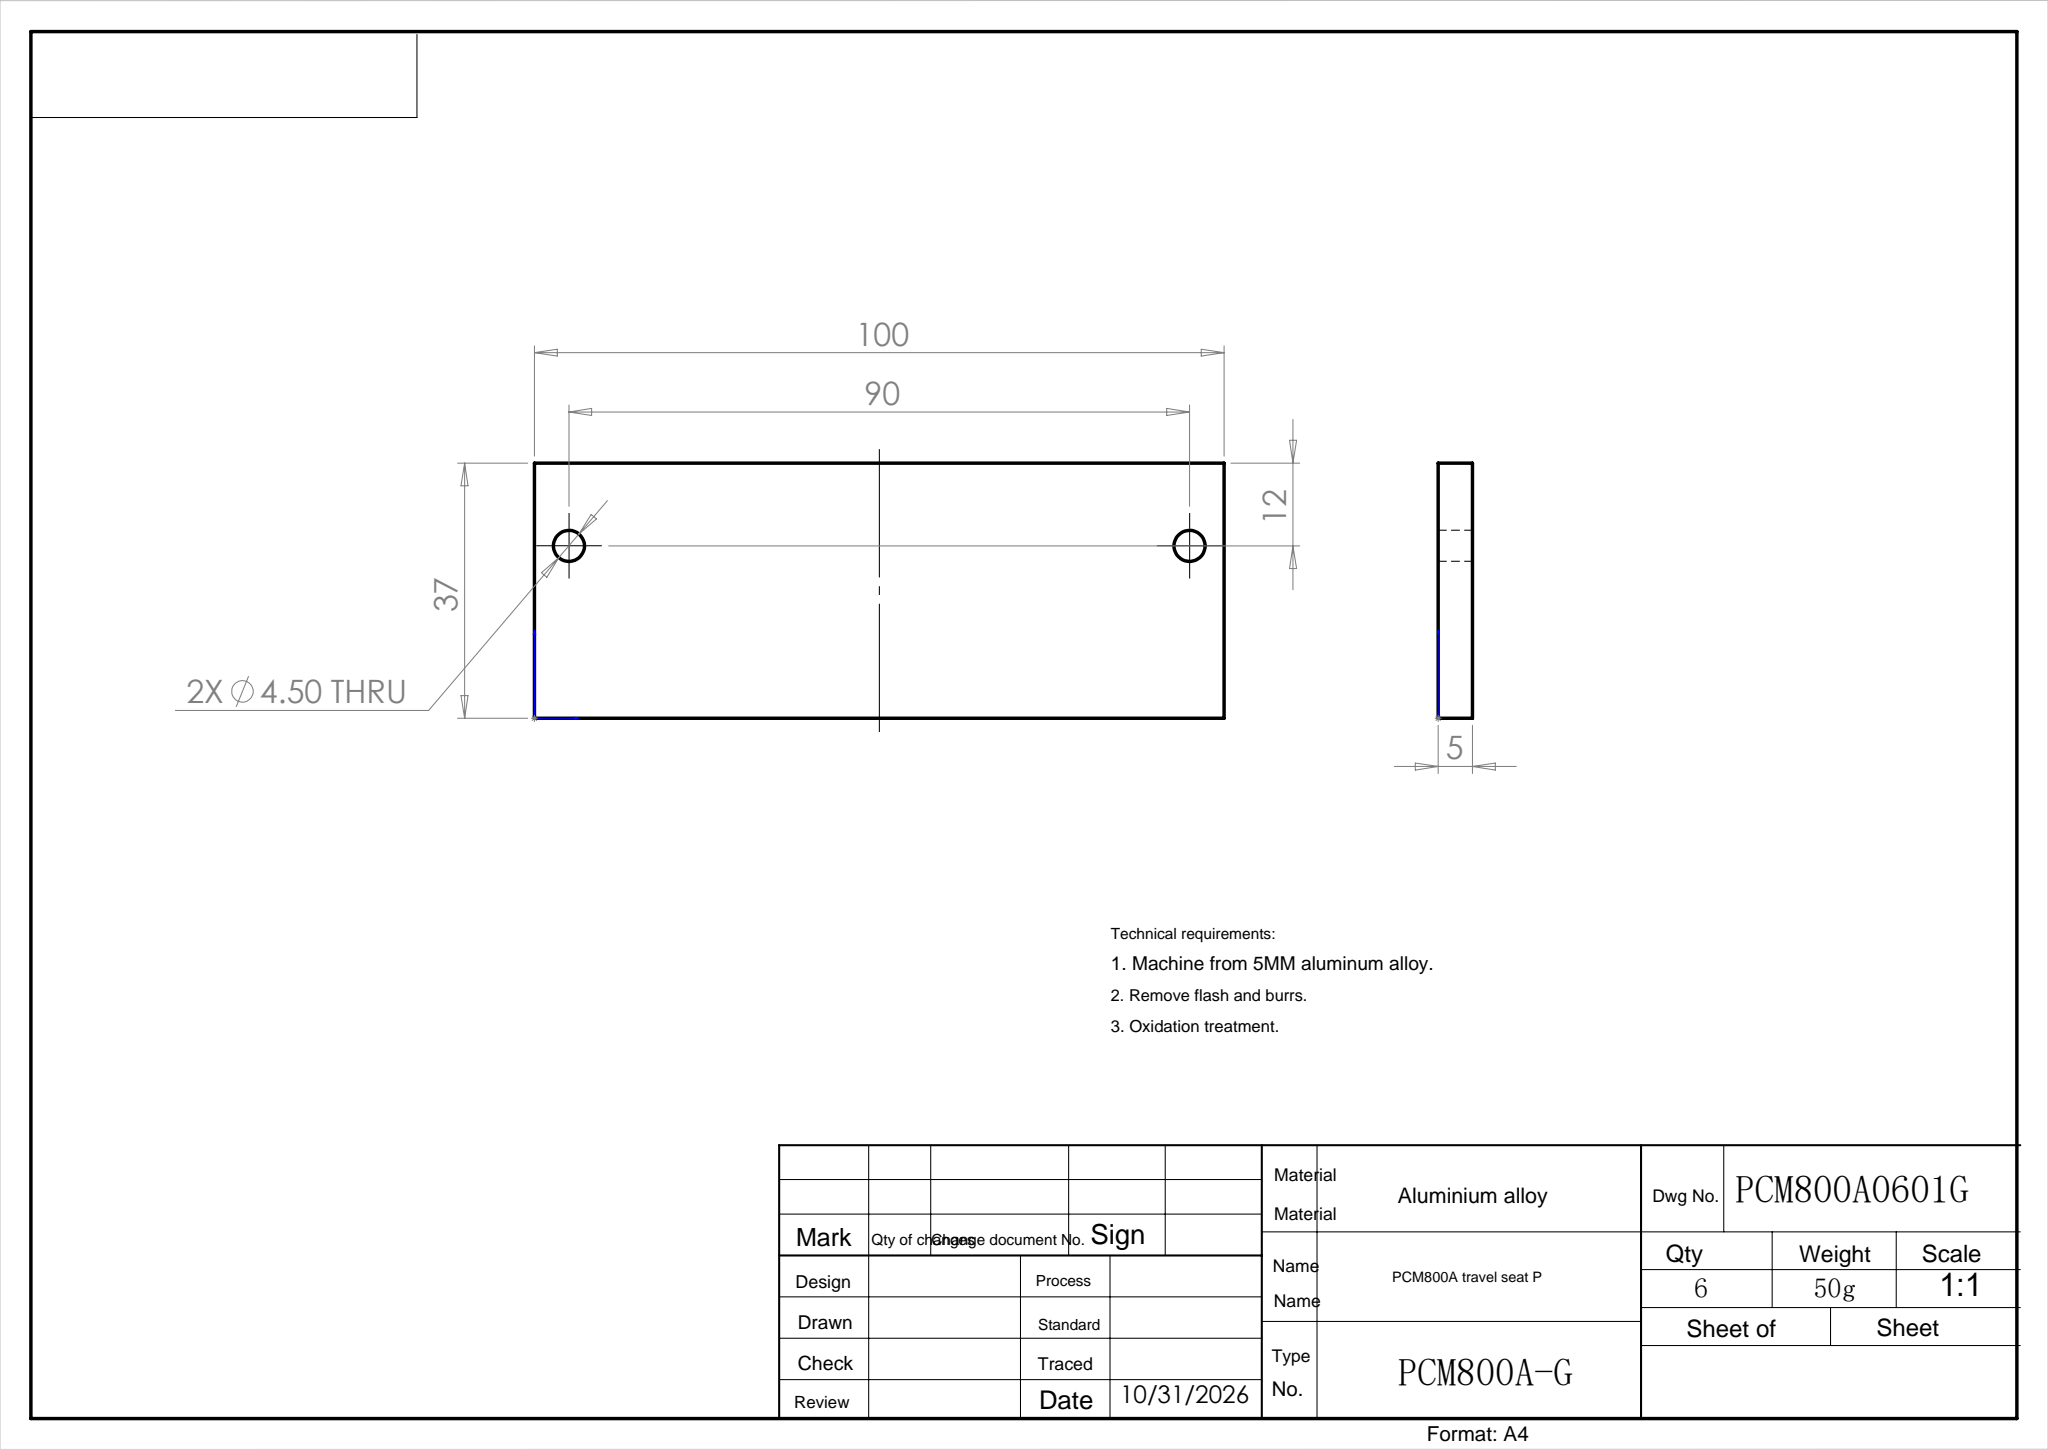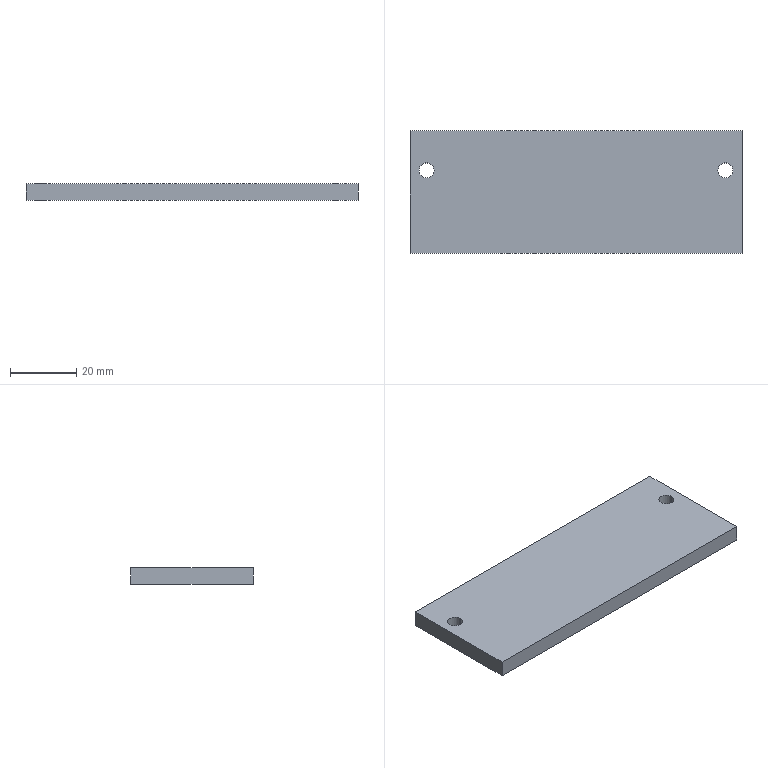Part | SolidWorks | features Extrusion 1, ICE 1 | 1 solid | 10 faces | box 100 x 37 x 5 mm | volume 18341 mm3 | plane 6 | cylinder 4 | commonest cylinder face diameters 4.5 x4
STEP:
#1=CARTESIAN_POINT('',(92.75,25.,0.));
#2=VERTEX_POINT('',#1);
#3=CARTESIAN_POINT('',(97.25,25.,0.));
#4=VERTEX_POINT('',#3);
#5=CARTESIAN_POINT('',(95.,25.,0.));
#6=DIRECTION('',(0.,0.,1.));
#7=DIRECTION('',(1.,0.,0.));
#8=AXIS2_PLACEMENT_3D('',#5,#6,#7);
#9=CIRCLE('',#8,2.25);
#10=EDGE_CURVE('',#2,#4,#9,.T.);
#11=ORIENTED_EDGE('',*,*,#10,.F.);
#12=CARTESIAN_POINT('',(92.75,25.,5.));
#13=VERTEX_POINT('',#12);
#14=CARTESIAN_POINT('',(92.75,25.,0.));
#15=DIRECTION('',(0.,0.,1.));
#16=VECTOR('',#15,1000.);
#17=LINE('',#14,#16);
#18=EDGE_CURVE('',#2,#13,#17,.T.);
#19=ORIENTED_EDGE('',*,*,#18,.T.);
#20=CARTESIAN_POINT('',(97.25,25.,5.));
#21=VERTEX_POINT('',#20);
#22=CARTESIAN_POINT('',(95.,25.,5.));
#23=DIRECTION('',(0.,0.,1.));
#24=DIRECTION('',(1.,0.,0.));
#25=AXIS2_PLACEMENT_3D('',#22,#23,#24);
#26=CIRCLE('',#25,2.25);
#27=EDGE_CURVE('',#13,#21,#26,.T.);
#28=ORIENTED_EDGE('',*,*,#27,.T.);
#29=CARTESIAN_POINT('',(97.25,25.,0.));
#30=DIRECTION('',(0.,0.,1.));
#31=VECTOR('',#30,1000.);
#32=LINE('',#29,#31);
#33=EDGE_CURVE('',#4,#21,#32,.T.);
#34=ORIENTED_EDGE('',*,*,#33,.F.);
#35=EDGE_LOOP('',(#11,#19,#28,#34));
#36=FACE_OUTER_BOUND('',#35,.T.);
#37=CARTESIAN_POINT('',(95.,25.,0.));
#38=DIRECTION('',(0.,0.,1.));
#39=DIRECTION('',(1.,0.,0.));
#40=AXIS2_PLACEMENT_3D('',#37,#38,#39);
#41=CYLINDRICAL_SURFACE('',#40,2.25);
#42=ADVANCED_FACE('',(#36),#41,.F.);
#43=CARTESIAN_POINT('',(2.75,25.,0.));
#44=VERTEX_POINT('',#43);
#45=CARTESIAN_POINT('',(7.25,25.,0.));
#46=VERTEX_POINT('',#45);
#47=CARTESIAN_POINT('',(5.,25.,0.));
#48=DIRECTION('',(0.,0.,1.));
#49=DIRECTION('',(1.,0.,0.));
#50=AXIS2_PLACEMENT_3D('',#47,#48,#49);
#51=CIRCLE('',#50,2.25);
#52=EDGE_CURVE('',#44,#46,#51,.T.);
#53=ORIENTED_EDGE('',*,*,#52,.F.);
#54=CARTESIAN_POINT('',(2.75,25.,5.));
#55=VERTEX_POINT('',#54);
#56=CARTESIAN_POINT('',(2.75,25.,0.));
#57=DIRECTION('',(0.,0.,1.));
#58=VECTOR('',#57,1000.);
#59=LINE('',#56,#58);
#60=EDGE_CURVE('',#44,#55,#59,.T.);
#61=ORIENTED_EDGE('',*,*,#60,.T.);
#62=CARTESIAN_POINT('',(7.25,25.,5.));
#63=VERTEX_POINT('',#62);
#64=CARTESIAN_POINT('',(5.,25.,5.));
#65=DIRECTION('',(0.,0.,1.));
#66=DIRECTION('',(1.,0.,0.));
#67=AXIS2_PLACEMENT_3D('',#64,#65,#66);
#68=CIRCLE('',#67,2.25);
#69=EDGE_CURVE('',#55,#63,#68,.T.);
#70=ORIENTED_EDGE('',*,*,#69,.T.);
#71=CARTESIAN_POINT('',(7.25,25.,0.));
#72=DIRECTION('',(0.,0.,1.));
#73=VECTOR('',#72,1000.);
#74=LINE('',#71,#73);
#75=EDGE_CURVE('',#46,#63,#74,.T.);
#76=ORIENTED_EDGE('',*,*,#75,.F.);
#77=EDGE_LOOP('',(#53,#61,#70,#76));
#78=FACE_OUTER_BOUND('',#77,.T.);
#79=CARTESIAN_POINT('',(5.,25.,0.));
#80=DIRECTION('',(0.,0.,1.));
#81=DIRECTION('',(1.,0.,0.));
#82=AXIS2_PLACEMENT_3D('',#79,#80,#81);
#83=CYLINDRICAL_SURFACE('',#82,2.25);
#84=ADVANCED_FACE('',(#78),#83,.F.);
#85=CARTESIAN_POINT('',(0.,37.,0.));
#86=VERTEX_POINT('',#85);
#87=CARTESIAN_POINT('',(0.,0.,0.));
#88=VERTEX_POINT('',#87);
#89=CARTESIAN_POINT('',(0.,0.,0.));
#90=DIRECTION('',(0.,-1.,0.));
#91=VECTOR('',#90,1000.);
#92=LINE('',#89,#91);
#93=EDGE_CURVE('',#86,#88,#92,.T.);
#94=ORIENTED_EDGE('',*,*,#93,.T.);
#95=CARTESIAN_POINT('',(0.,0.,5.));
#96=VERTEX_POINT('',#95);
#97=CARTESIAN_POINT('',(0.,0.,5.));
#98=DIRECTION('',(0.,0.,-1.));
#99=VECTOR('',#98,1000.);
#100=LINE('',#97,#99);
#101=EDGE_CURVE('',#96,#88,#100,.T.);
#102=ORIENTED_EDGE('',*,*,#101,.F.);
#103=CARTESIAN_POINT('',(0.,37.,5.));
#104=VERTEX_POINT('',#103);
#105=CARTESIAN_POINT('',(0.,0.,5.));
#106=DIRECTION('',(0.,-1.,0.));
#107=VECTOR('',#106,1000.);
#108=LINE('',#105,#107);
#109=EDGE_CURVE('',#104,#96,#108,.T.);
#110=ORIENTED_EDGE('',*,*,#109,.F.);
#111=CARTESIAN_POINT('',(0.,37.,5.));
#112=DIRECTION('',(0.,0.,-1.));
#113=VECTOR('',#112,1000.);
#114=LINE('',#111,#113);
#115=EDGE_CURVE('',#104,#86,#114,.T.);
#116=ORIENTED_EDGE('',*,*,#115,.T.);
#117=EDGE_LOOP('',(#94,#102,#110,#116));
#118=FACE_OUTER_BOUND('',#117,.T.);
#119=CARTESIAN_POINT('',(0.,0.,5.));
#120=DIRECTION('',(1.,0.,0.));
#121=DIRECTION('',(0.,0.,-1.));
#122=AXIS2_PLACEMENT_3D('',#119,#120,#121);
#123=PLANE('',#122);
#124=ADVANCED_FACE('',(#118),#123,.F.);
#125=CARTESIAN_POINT('',(100.,0.,0.));
#126=VERTEX_POINT('',#125);
#127=CARTESIAN_POINT('',(0.,0.,0.));
#128=DIRECTION('',(1.,0.,0.));
#129=VECTOR('',#128,1000.);
#130=LINE('',#127,#129);
#131=EDGE_CURVE('',#88,#126,#130,.T.);
#132=ORIENTED_EDGE('',*,*,#131,.T.);
#133=CARTESIAN_POINT('',(100.,0.,5.));
#134=VERTEX_POINT('',#133);
#135=CARTESIAN_POINT('',(100.,0.,5.));
#136=DIRECTION('',(0.,0.,-1.));
#137=VECTOR('',#136,1000.);
#138=LINE('',#135,#137);
#139=EDGE_CURVE('',#134,#126,#138,.T.);
#140=ORIENTED_EDGE('',*,*,#139,.F.);
#141=CARTESIAN_POINT('',(0.,0.,5.));
#142=DIRECTION('',(1.,0.,0.));
#143=VECTOR('',#142,1000.);
#144=LINE('',#141,#143);
#145=EDGE_CURVE('',#96,#134,#144,.T.);
#146=ORIENTED_EDGE('',*,*,#145,.F.);
#147=ORIENTED_EDGE('',*,*,#101,.T.);
#148=EDGE_LOOP('',(#132,#140,#146,#147));
#149=FACE_OUTER_BOUND('',#148,.T.);
#150=CARTESIAN_POINT('',(0.,0.,5.));
#151=DIRECTION('',(0.,1.,0.));
#152=DIRECTION('',(0.,0.,1.));
#153=AXIS2_PLACEMENT_3D('',#150,#151,#152);
#154=PLANE('',#153);
#155=ADVANCED_FACE('',(#149),#154,.F.);
#156=CARTESIAN_POINT('',(100.,37.,0.));
#157=VERTEX_POINT('',#156);
#158=CARTESIAN_POINT('',(100.,0.,0.));
#159=DIRECTION('',(0.,1.,0.));
#160=VECTOR('',#159,1000.);
#161=LINE('',#158,#160);
#162=EDGE_CURVE('',#126,#157,#161,.T.);
#163=ORIENTED_EDGE('',*,*,#162,.T.);
#164=CARTESIAN_POINT('',(100.,37.,5.));
#165=VERTEX_POINT('',#164);
#166=CARTESIAN_POINT('',(100.,37.,5.));
#167=DIRECTION('',(0.,0.,-1.));
#168=VECTOR('',#167,1000.);
#169=LINE('',#166,#168);
#170=EDGE_CURVE('',#165,#157,#169,.T.);
#171=ORIENTED_EDGE('',*,*,#170,.F.);
#172=CARTESIAN_POINT('',(100.,0.,5.));
#173=DIRECTION('',(0.,1.,0.));
#174=VECTOR('',#173,1000.);
#175=LINE('',#172,#174);
#176=EDGE_CURVE('',#134,#165,#175,.T.);
#177=ORIENTED_EDGE('',*,*,#176,.F.);
#178=ORIENTED_EDGE('',*,*,#139,.T.);
#179=EDGE_LOOP('',(#163,#171,#177,#178));
#180=FACE_OUTER_BOUND('',#179,.T.);
#181=CARTESIAN_POINT('',(100.,0.,5.));
#182=DIRECTION('',(-1.,0.,0.));
#183=DIRECTION('',(0.,0.,1.));
#184=AXIS2_PLACEMENT_3D('',#181,#182,#183);
#185=PLANE('',#184);
#186=ADVANCED_FACE('',(#180),#185,.F.);
#187=CARTESIAN_POINT('',(0.,37.,0.));
#188=DIRECTION('',(-1.,0.,0.));
#189=VECTOR('',#188,1000.);
#190=LINE('',#187,#189);
#191=EDGE_CURVE('',#157,#86,#190,.T.);
#192=ORIENTED_EDGE('',*,*,#191,.T.);
#193=ORIENTED_EDGE('',*,*,#115,.F.);
#194=CARTESIAN_POINT('',(0.,37.,5.));
#195=DIRECTION('',(-1.,0.,0.));
#196=VECTOR('',#195,1000.);
#197=LINE('',#194,#196);
#198=EDGE_CURVE('',#165,#104,#197,.T.);
#199=ORIENTED_EDGE('',*,*,#198,.F.);
#200=ORIENTED_EDGE('',*,*,#170,.T.);
#201=EDGE_LOOP('',(#192,#193,#199,#200));
#202=FACE_OUTER_BOUND('',#201,.T.);
#203=CARTESIAN_POINT('',(0.,37.,5.));
#204=DIRECTION('',(0.,-1.,0.));
#205=DIRECTION('',(0.,0.,-1.));
#206=AXIS2_PLACEMENT_3D('',#203,#204,#205);
#207=PLANE('',#206);
#208=ADVANCED_FACE('',(#202),#207,.F.);
#209=CARTESIAN_POINT('',(95.,25.,5.));
#210=DIRECTION('',(0.,0.,1.));
#211=DIRECTION('',(1.,0.,0.));
#212=AXIS2_PLACEMENT_3D('',#209,#210,#211);
#213=CIRCLE('',#212,2.25);
#214=EDGE_CURVE('',#21,#13,#213,.T.);
#215=ORIENTED_EDGE('',*,*,#214,.F.);
#216=ORIENTED_EDGE('',*,*,#27,.F.);
#217=EDGE_LOOP('',(#215,#216));
#218=FACE_BOUND('',#217,.T.);
#219=CARTESIAN_POINT('',(5.,25.,5.));
#220=DIRECTION('',(0.,0.,1.));
#221=DIRECTION('',(1.,0.,0.));
#222=AXIS2_PLACEMENT_3D('',#219,#220,#221);
#223=CIRCLE('',#222,2.25);
#224=EDGE_CURVE('',#63,#55,#223,.T.);
#225=ORIENTED_EDGE('',*,*,#224,.F.);
#226=ORIENTED_EDGE('',*,*,#69,.F.);
#227=EDGE_LOOP('',(#225,#226));
#228=FACE_BOUND('',#227,.T.);
#229=ORIENTED_EDGE('',*,*,#109,.T.);
#230=ORIENTED_EDGE('',*,*,#145,.T.);
#231=ORIENTED_EDGE('',*,*,#176,.T.);
#232=ORIENTED_EDGE('',*,*,#198,.T.);
#233=EDGE_LOOP('',(#229,#230,#231,#232));
#234=FACE_OUTER_BOUND('',#233,.T.);
#235=CARTESIAN_POINT('',(0.,37.,5.));
#236=DIRECTION('',(0.,0.,-1.));
#237=DIRECTION('',(-1.,0.,0.));
#238=AXIS2_PLACEMENT_3D('',#235,#236,#237);
#239=PLANE('',#238);
#240=ADVANCED_FACE('',(#218,#228,#234),#239,.F.);
#241=CARTESIAN_POINT('',(95.,25.,0.));
#242=DIRECTION('',(0.,0.,1.));
#243=DIRECTION('',(1.,0.,0.));
#244=AXIS2_PLACEMENT_3D('',#241,#242,#243);
#245=CIRCLE('',#244,2.25);
#246=EDGE_CURVE('',#4,#2,#245,.T.);
#247=ORIENTED_EDGE('',*,*,#246,.T.);
#248=ORIENTED_EDGE('',*,*,#10,.T.);
#249=EDGE_LOOP('',(#247,#248));
#250=FACE_BOUND('',#249,.T.);
#251=CARTESIAN_POINT('',(5.,25.,0.));
#252=DIRECTION('',(0.,0.,1.));
#253=DIRECTION('',(1.,0.,0.));
#254=AXIS2_PLACEMENT_3D('',#251,#252,#253);
#255=CIRCLE('',#254,2.25);
#256=EDGE_CURVE('',#46,#44,#255,.T.);
#257=ORIENTED_EDGE('',*,*,#256,.T.);
#258=ORIENTED_EDGE('',*,*,#52,.T.);
#259=EDGE_LOOP('',(#257,#258));
#260=FACE_BOUND('',#259,.T.);
#261=ORIENTED_EDGE('',*,*,#93,.F.);
#262=ORIENTED_EDGE('',*,*,#191,.F.);
#263=ORIENTED_EDGE('',*,*,#162,.F.);
#264=ORIENTED_EDGE('',*,*,#131,.F.);
#265=EDGE_LOOP('',(#261,#262,#263,#264));
#266=FACE_OUTER_BOUND('',#265,.T.);
#267=CARTESIAN_POINT('',(0.,37.,0.));
#268=DIRECTION('',(0.,0.,-1.));
#269=DIRECTION('',(-1.,0.,0.));
#270=AXIS2_PLACEMENT_3D('',#267,#268,#269);
#271=PLANE('',#270);
#272=ADVANCED_FACE('',(#250,#260,#266),#271,.T.);
#273=ORIENTED_EDGE('',*,*,#60,.F.);
#274=ORIENTED_EDGE('',*,*,#256,.F.);
#275=ORIENTED_EDGE('',*,*,#75,.T.);
#276=ORIENTED_EDGE('',*,*,#224,.T.);
#277=EDGE_LOOP('',(#273,#274,#275,#276));
#278=FACE_OUTER_BOUND('',#277,.T.);
#279=CARTESIAN_POINT('',(5.,25.,0.));
#280=DIRECTION('',(0.,0.,1.));
#281=DIRECTION('',(1.,0.,0.));
#282=AXIS2_PLACEMENT_3D('',#279,#280,#281);
#283=CYLINDRICAL_SURFACE('',#282,2.25);
#284=ADVANCED_FACE('',(#278),#283,.F.);
#285=ORIENTED_EDGE('',*,*,#18,.F.);
#286=ORIENTED_EDGE('',*,*,#246,.F.);
#287=ORIENTED_EDGE('',*,*,#33,.T.);
#288=ORIENTED_EDGE('',*,*,#214,.T.);
#289=EDGE_LOOP('',(#285,#286,#287,#288));
#290=FACE_OUTER_BOUND('',#289,.T.);
#291=CARTESIAN_POINT('',(95.,25.,0.));
#292=DIRECTION('',(0.,0.,1.));
#293=DIRECTION('',(1.,0.,0.));
#294=AXIS2_PLACEMENT_3D('',#291,#292,#293);
#295=CYLINDRICAL_SURFACE('',#294,2.25);
#296=ADVANCED_FACE('',(#290),#295,.F.);
#297=CLOSED_SHELL('',(#42,#84,#124,#155,#186,#208,#240,#272,#284,#296));
#298=MANIFOLD_SOLID_BREP('',#297);
#299=CARTESIAN_POINT('',(0.,0.,0.));
#300=DIRECTION('',(0.,0.,1.));
#301=DIRECTION('',(1.,0.,0.));
#302=AXIS2_PLACEMENT_3D('',#299,#300,#301);
#303=(LENGTH_UNIT()NAMED_UNIT(*)SI_UNIT(.MILLI.,.METRE.));
#304=UNCERTAINTY_MEASURE_WITH_UNIT(LENGTH_MEASURE(0.00001),#303,'','');
#305=(NAMED_UNIT(*)PLANE_ANGLE_UNIT()SI_UNIT($,.RADIAN.));
#306=(NAMED_UNIT(*)SI_UNIT($,.STERADIAN.)SOLID_ANGLE_UNIT());
#307=(GEOMETRIC_REPRESENTATION_CONTEXT(3)GLOBAL_UNCERTAINTY_ASSIGNED_CONTEXT((#304))GLOBAL_UNIT_ASSIGNED_CONTEXT((#303,#305,#306))REPRESENTATION_CONTEXT('',''));
#308=ADVANCED_BREP_SHAPE_REPRESENTATION('',(#298,#302),#307);